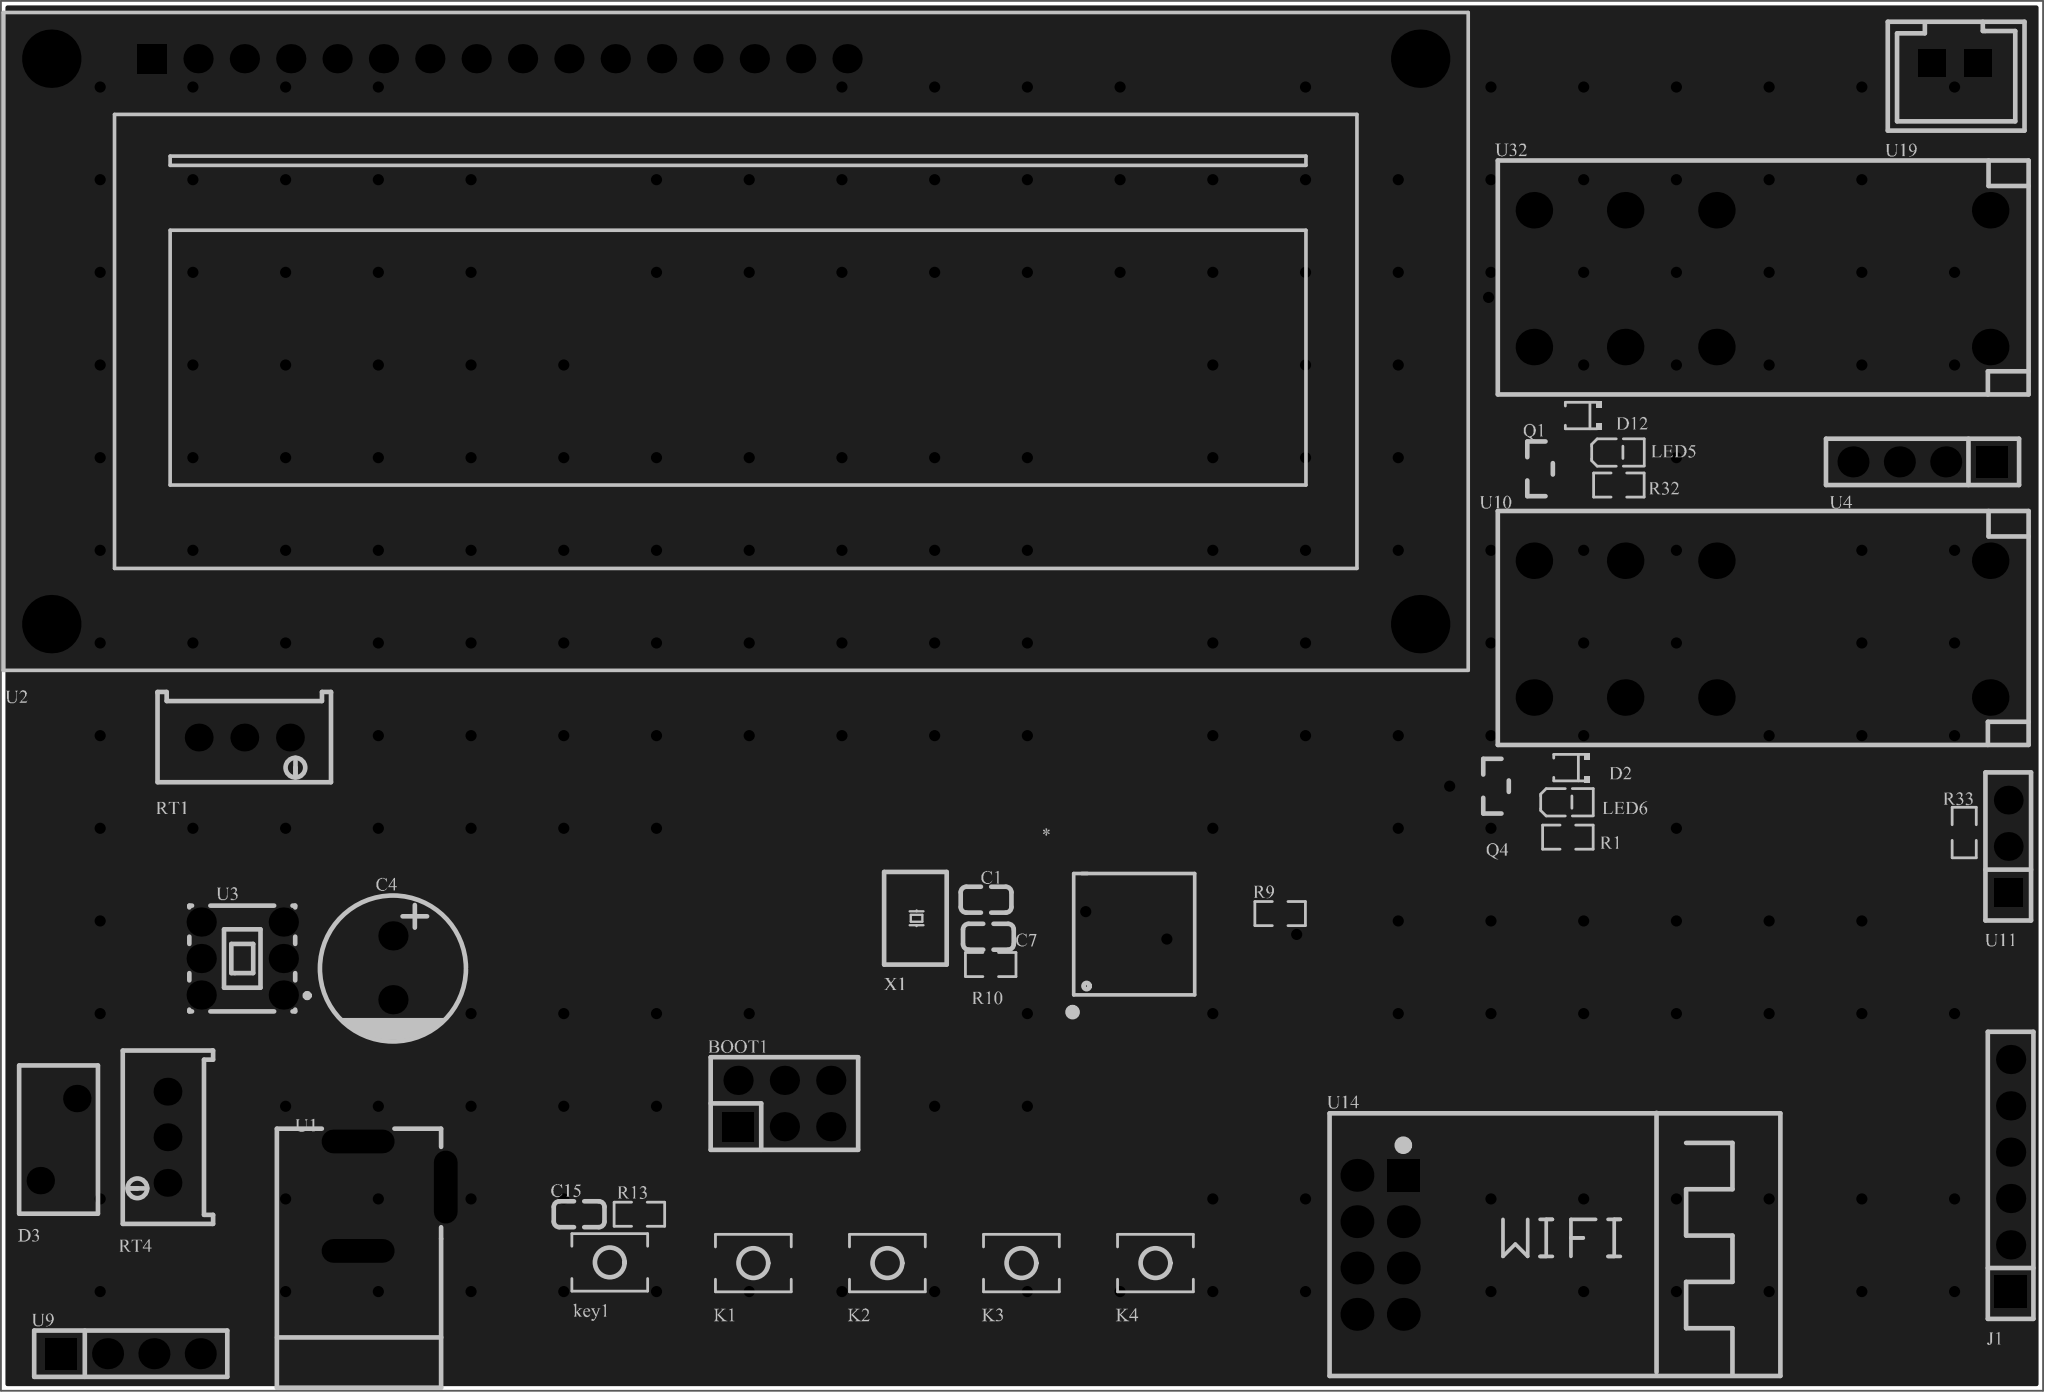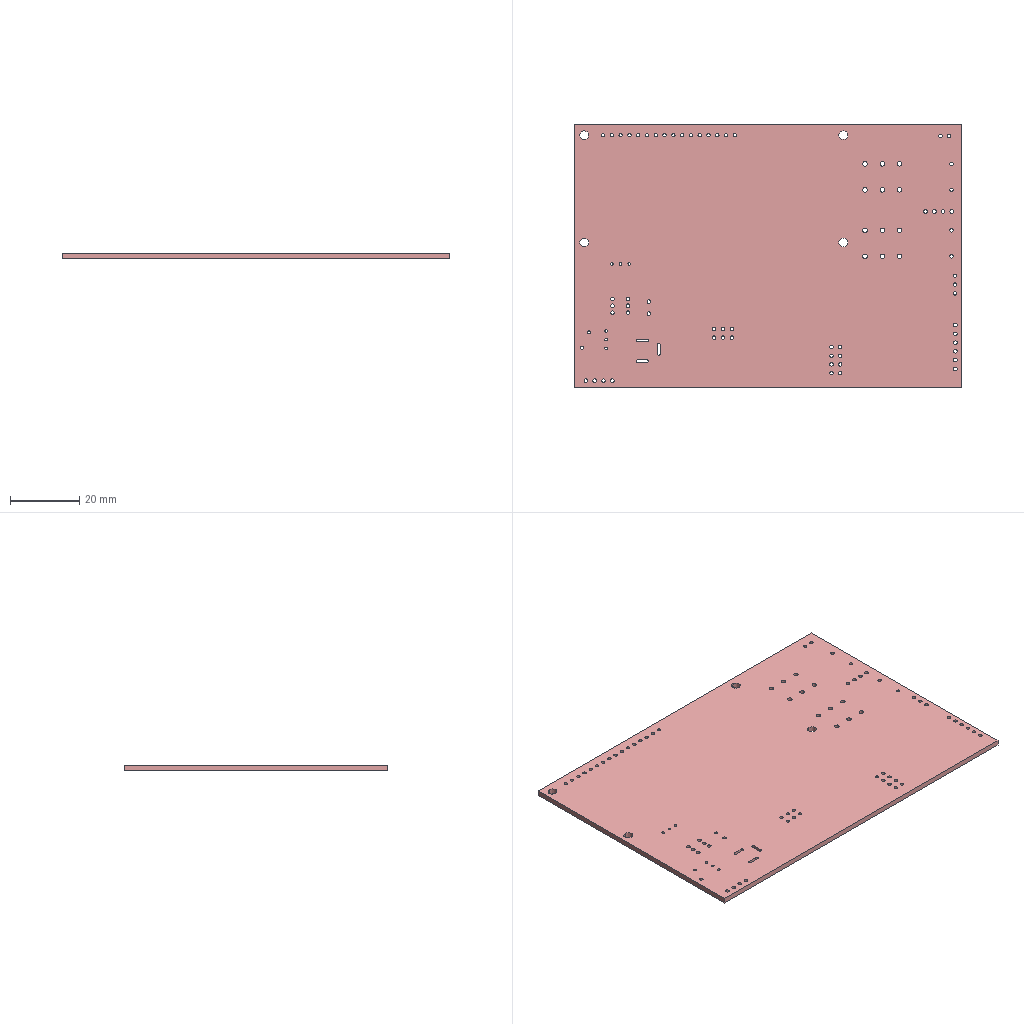Circuit board layout | Altium Designer | box 111.9 x 76.2 x 1.6 mm
Layer stack:
# Altium Designer layer stack of  (unit mm; dielectric type: 0 none, 1 core, 2 prepreg, 3 surface material)
index,name,kind,layer,copper_thickness_mm,dielectric_type,dielectric_thickness_mm,dielectric_material,dielectric_constant
0,Top Paste Mask Layer,other,,,,,,
1,Top Silkscreen Layer,other,,,,,,
2,Top Solder Mask Layer,dielectric,,,3,0.01,,3.3
3,Top Layer,copper,Top Layer,0.035,,,,
4,Dielectric1,dielectric,,,3,1.51,FR4,4.5
5,Bottom Layer,copper,Bottom Layer,0.035,,,,
6,Bottom Solder Mask Layer,dielectric,,,3,0.01,,3.3
7,Bottom Silkscreen Layer,other,,,,,,
8,Bottom Paste Mask Layer,other,,,,,,
# drill layer pairs: low layer,high layer
drill_pair,Top Layer,Bottom Layer
Part placement:
Designator,Comment,Layer,Footprint,Center-X(mm),Center-Y(mm),Rotation
*,程序下载口,TopLayer,LQFP-48_L7.0-W7.0-P0.50-LS9.0-BL,141.097,108.966,0
BOOT1,Header 3X2,TopLayer,HDR-TH_6P-P2.54-V-F-R2-C3-S2.54,121.92,99.695,0
C1,20pF,TopLayer,C0603,132.969,110.871,0
C4,1000UF,TopLayer,CAP-TH_BD8.0-P3.50-D0.6-FD_1,100.472,107.137,270
C7,20pF,TopLayer,C0603,133.096,108.839,0
C15,104,TopLayer,C0603,110.673,93.626,0
D2,IN4148,TopLayer,SOD-323_L1.8-W1.3-LS2.5-RD,164.973,118.11,180
D3,光敏电阻,TopLayer,RES-TH_L8.0-W4.4-P4.50-D0.6-S2.0,82.151,97.719,90
D12,IN4148,TopLayer,SOD-323_L1.8-W1.3-LS2.5-RD,165.608,137.414,180
J1,,TopLayer,HDR-TH_6P-P2.54-V-F,189.103,95.758,90
K1,,TopLayer,Key_SMD_3x4x2,120.218,90.947,180
K2,,TopLayer,Key_SMD_3x4x2,127.562,90.947,180
K3,,TopLayer,Key_SMD_3x4x2,134.906,90.947,180
K4,,TopLayer,Key_SMD_3x4x2,142.249,90.947,180
key1,KEY_M,TopLayer,Key_SMD_3x4x2,112.352,90.985,180
LED5,LED,TopLayer,LED0603,167.64,135.382,0
LED6,LED,TopLayer,LED0603,164.846,116.205,0
Q1,S8050,TopLayer,S8050_SOT-23,163.322,134.493,0
Q4,S8050,TopLayer,S8050_SOT-23,160.909,117.094,0
R1,1K,TopLayer,R0603,164.846,114.3,0
R9,10K,TopLayer,R0603,149.081,110.109,0
R10,10K,TopLayer,R0603,133.223,107.315,0
R13,10 K,TopLayer,R0603,113.975,93.626,180
R32,1K,TopLayer,R0603,167.64,133.604,0
R33,10K,TopLayer,R0603,186.56,114.551,90
RT1,10K,TopLayer,R_3296,92.329,119.761,180
RT4,10K,TopLayer,R_3296,88.12,97.846,90
U1,POW,TopLayer,DC-2.0,100.965,94.615,270
U2,LCD1602,TopLayer,LCD1602,119.253,141.478,0
U3,SWITCH,TopLayer,SW-TH_6P-L5.8-W5.8-P2.00-LS4.5-TR,92.217,107.645,270
U4,,TopLayer,HDR-TH_4P-P2.54-V-F,184.277,134.874,180
U9,,TopLayer,HDR-TH_4P-P2.54-V-F,86.106,85.979,0
U10,JDQ-5,TopLayer,RELAY-TH_FTR-K1CK024W,175.484,125.704,0
U11,DHT11,TopLayer,HDR-TH_3P-P2.54-V-F,188.973,113.789,90
U14,ESP8266,TopLayer,WIFIM-TH_8P-L24.7-W14.4-P2.54,154.559,91.948,0
U19,,TopLayer,CONN-TH_XH2.54-2P,186.055,156.718,180
U32,JDQ-5,TopLayer,RELAY-TH_FTR-K1CK024W,175.484,144.92,0
X1,8MHz,TopLayer,CRYSTAL-SMD_L3.2-W2.5_3225-8MHZ,129.161,109.852,90
Pad and via stacks:
# Altium Designer via and pad stacks of  (unit mm). Each distinct definition once, with the count of objects using it.
# via: kind,start_layer,end_layer,hole_mm,diameter_mm,mode(0 simple;1 top-mid-bottom;2 full stack),diameter_per_layer,count,example_net
# pad: kind,layer,hole_mm,hole_type(0 round;1 square;2 slot),plating,top_size,top_shape(1 round;2 rect;3 octagon;9 rounded rect),mid_size,bottom_size,mode,footprint,size_per_layer,count,example
pad,Top Layer,0,0,plated,0.27x1.5,1,0.27x1.5,0.27x1.5,0,LQFP-48_L7.0-W7.0-P0.50-LS9.0-BL,,24,*.1
pad,Top Layer,0,0,plated,1.5x0.27,1,1.5x0.27,1.5x0.27,0,LQFP-48_L7.0-W7.0-P0.50-LS9.0-BL,,24,*.13
pad,Top Layer,0,0,plated,0.8x0.9,2,0.8x0.9,0.8x0.9,0,C0603,,6,C1.2
pad,Top Layer,0,0,plated,1x0.7,2,1x0.7,1x0.7,0,SOD-323_L1.8-W1.3-LS2.5-RD,,4,D2.1
pad,Top Layer,0,0,plated,1.53x1.36,2,1.53x1.36,1.53x1.36,0,Key_SMD_3x4x2,,10,K1.1
pad,Top Layer,0,0,plated,0.8x0.8,2,0.8x0.8,0.8x0.8,0,LED0603,,4,LED5.2
pad,Top Layer,0,0,plated,1x0.8,2,1x0.8,1x0.8,0,S8050_SOT-23,,6,Q1.2
pad,Top Layer,0,0,plated,0.8065x0.864,2,0.8065x0.864,0.8065x0.864,0,R0603,,12,R1.2
pad,Top Layer,0,0,plated,1.524x2.7,2,1.524x2.7,1.524x2.7,0,CRYSTAL-SMD_L3.2-W2.5_3225-8MHZ,,2,X1.1
pad,Multi-Layer,1,0,plated,1.7x1.6,2,1.7x1.6,1.7x1.6,0,HDR-TH_6P-P2.54-V-F-R2-C3-S2.54,,1,BOOT1.1
pad,Multi-Layer,1,0,plated,1.6x1.6,1,1.6x1.6,1.6x1.6,0,HDR-TH_6P-P2.54-V-F-R2-C3-S2.54,,5,BOOT1.2
pad,Multi-Layer,1,0,plated,1.6x1.6,1,1.6x1.6,1.6x1.6,0,CAP-TH_BD8.0-P3.50-D0.6-FD_1,,2,C4.2
pad,Multi-Layer,0.9,0,plated,1.5x1.5,1,1.5x1.5,1.5x1.5,0,RES-TH_L8.0-W4.4-P4.50-D0.6-S2.0,,2,D3.1
pad,Multi-Layer,1.02,0,plated,1.6x1.6,1,1.6x1.6,1.6x1.6,0,HDR-TH_6P-P2.54-V-F,,5,J1.6
pad,Multi-Layer,1.02,0,plated,1.8x1.8,2,1.8x1.8,1.8x1.8,0,HDR-TH_6P-P2.54-V-F,,1,J1.1
pad,Multi-Layer,0.762,0,plated,1.524x1.524,1,1.524x1.524,1.524x1.524,0,R_3296,,6,RT1.2
pad,Multi-Layer,0.8001,2,plated,4x1.3,1,4x1.3,4x1.3,0,DC-2.0,,3,U1.2
pad,Multi-Layer,1,0,plated,1.6x1.6,1,1.6x1.6,1.6x1.6,0,LCD1602,,15,U2.16
pad,Multi-Layer,1,0,plated,1.6x1.6,2,1.6x1.6,1.6x1.6,0,LCD1602,,1,U2.1
pad,Multi-Layer,2.5,2,plated,3.2x3.2,1,3.2x3.2,3.2x3.2,0,LCD1602,,4,U2.0
pad,Multi-Layer,1.1,0,plated,1.6x1.6,1,1.6x1.6,1.6x1.6,0,SW-TH_6P-L5.8-W5.8-P2.00-LS4.5-TR,,6,U3.6
pad,Multi-Layer,1.1,0,plated,1.7x1.7,2,1.7x1.7,1.7x1.7,0,HDR-TH_4P-P2.54-V-F,,2,U4.1
pad,Multi-Layer,1.1,0,plated,1.7x1.7,1,1.7x1.7,1.7x1.7,0,HDR-TH_4P-P2.54-V-F,,6,U4.2
pad,Multi-Layer,1.3,0,plated,2x2,1,2x2,2x2,0,RELAY-TH_FTR-K1CK024W,,12,U10.8
pad,Multi-Layer,1,0,plated,2x2,1,2x2,2x2,0,RELAY-TH_FTR-K1CK024W,,4,U10.5
pad,Multi-Layer,1.02,0,plated,1.575x1.575,1,1.575x1.575,1.575x1.575,0,HDR-TH_3P-P2.54-V-F,,2,U11.3
pad,Multi-Layer,1.02,0,plated,1.575x1.575,2,1.575x1.575,1.575x1.575,0,HDR-TH_3P-P2.54-V-F,,1,U11.1
pad,Multi-Layer,1,0,plated,1.8x1.8,1,1.8x1.8,1.8x1.8,0,WIFIM-TH_8P-L24.7-W14.4-P2.54,,7,U14.8
pad,Multi-Layer,1,0,plated,1.8x1.8,2,1.8x1.8,1.8x1.8,0,WIFIM-TH_8P-L24.7-W14.4-P2.54,,1,U14.1
pad,Multi-Layer,1,2,plated,1.524x1.524,2,1.524x1.524,1.524x1.524,0,CONN-TH_XH2.54-2P,,2,U19.1
via,Top Layer,Bottom Layer,0.3048,0.61,0,,213,$2N54
Copper pours:
name,layer,net,type(0 solid;1 hatched;2 none)
Top Layer-GND,Top Layer,GND,0
Bottom Layer-GND,Bottom Layer,GND,0